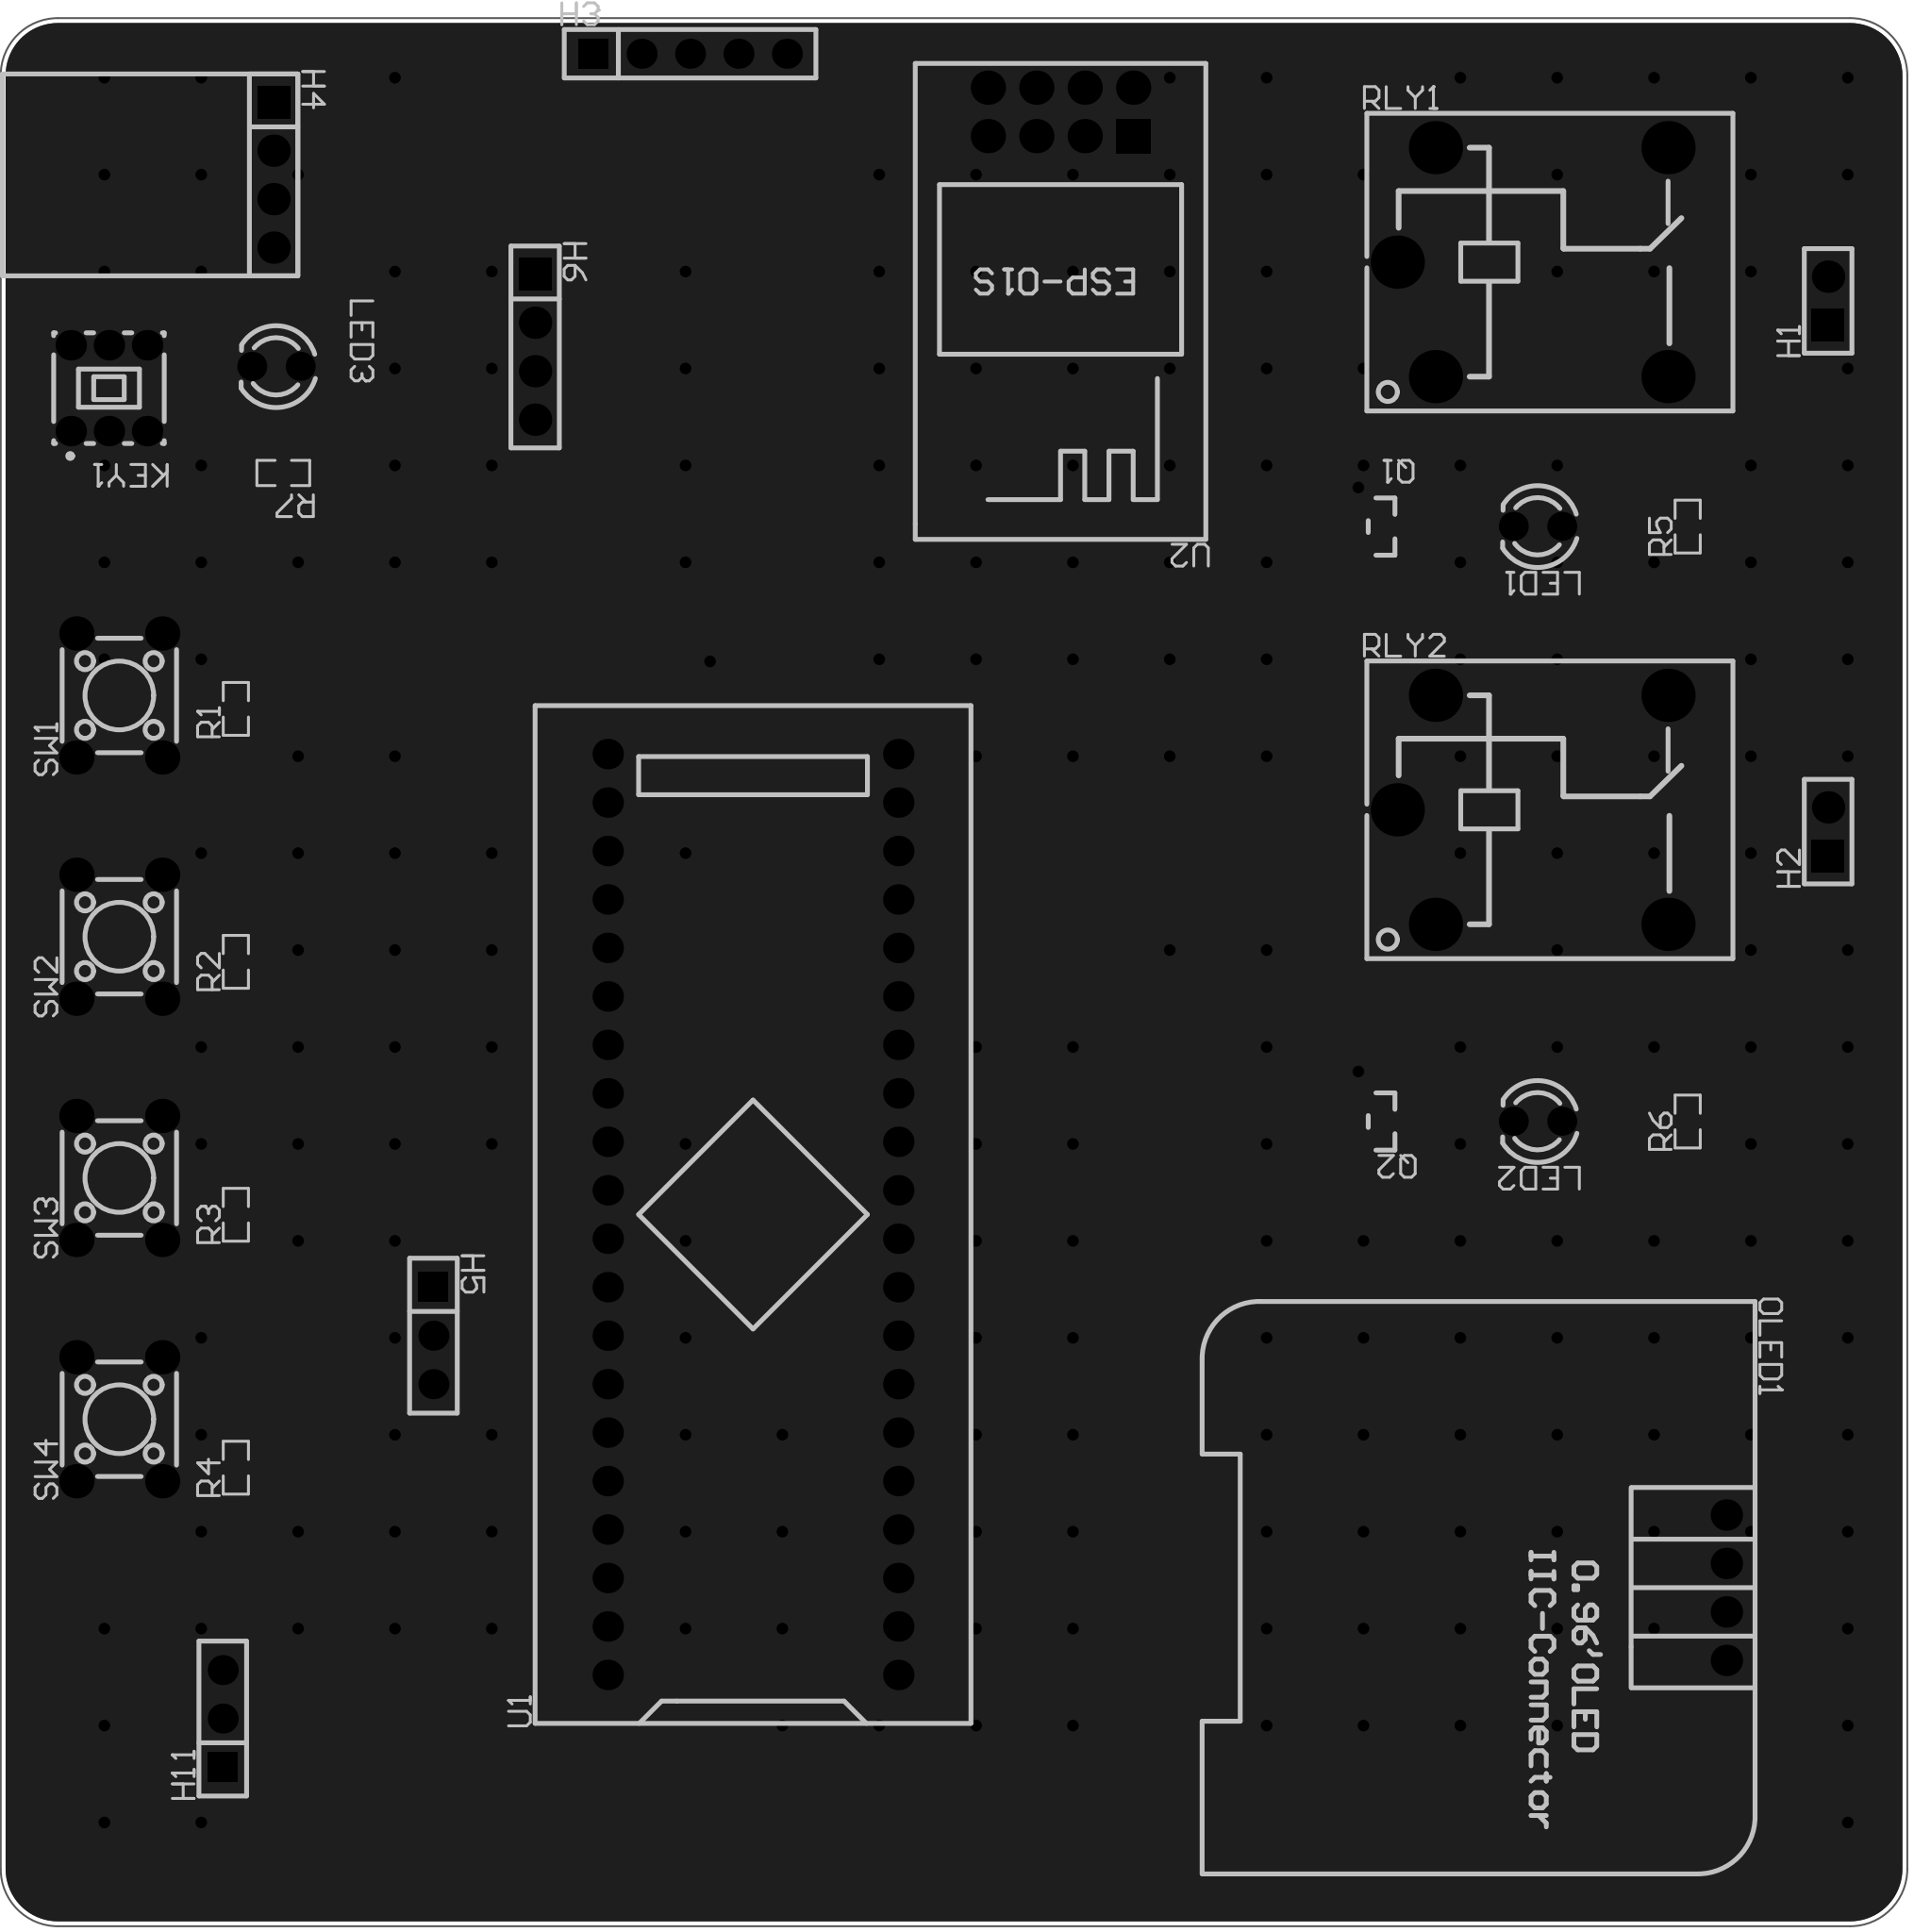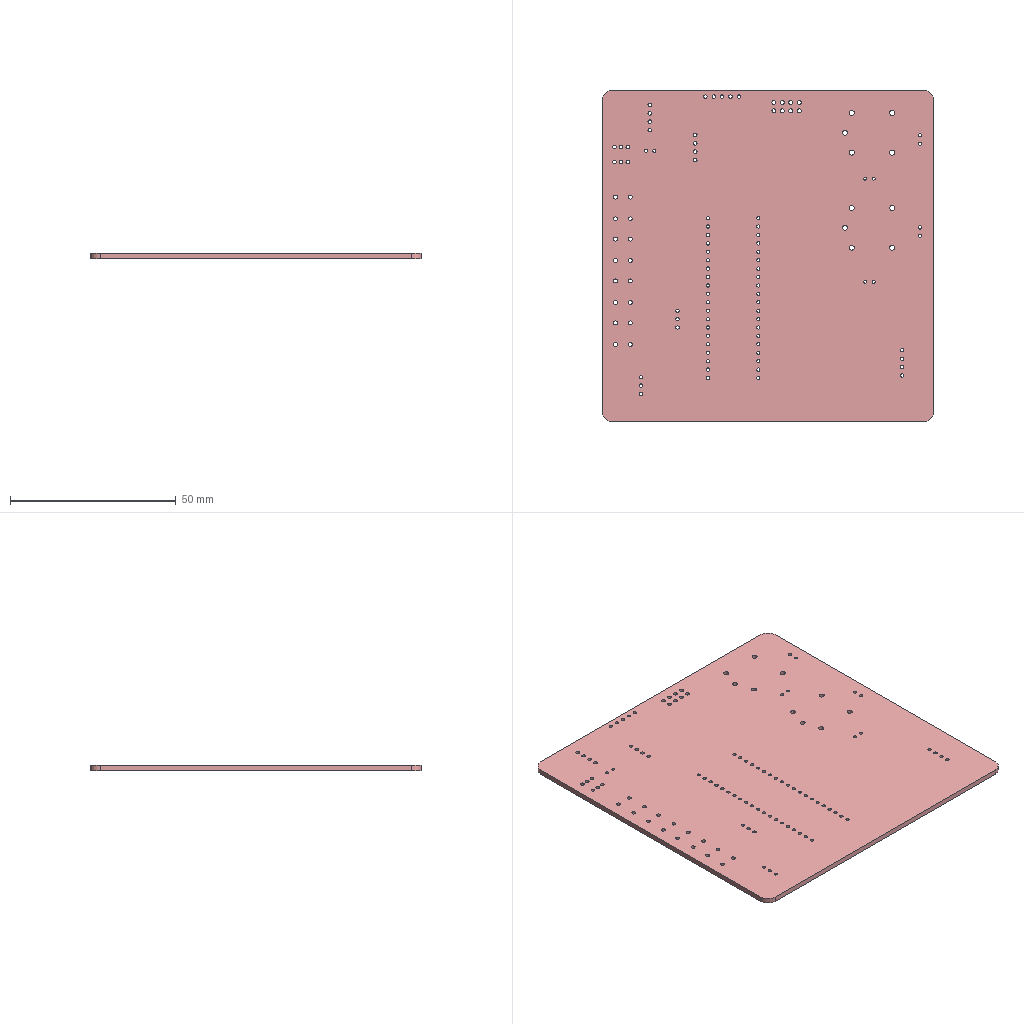Circuit board layout | Altium Designer | box 100 x 100 x 1.6 mm
Layer stack:
# Altium Designer layer stack of  (unit mm; dielectric type: 0 none, 1 core, 2 prepreg, 3 surface material)
index,name,kind,layer,copper_thickness_mm,dielectric_type,dielectric_thickness_mm,dielectric_material,dielectric_constant
0,Top Paste Mask Layer,other,,,,,,
1,Top Silkscreen Layer,other,,,,,,
2,Top Solder Mask Layer,dielectric,,,3,0.01,,3.3
3,Top Layer,copper,Top Layer,0.035,,,,
4,Dielectric1,dielectric,,,3,1.51,FR4,4.5
5,Bottom Layer,copper,Bottom Layer,0.035,,,,
6,Bottom Solder Mask Layer,dielectric,,,3,0.01,,3.3
7,Bottom Silkscreen Layer,other,,,,,,
8,Bottom Paste Mask Layer,other,,,,,,
# drill layer pairs: low layer,high layer
drill_pair,Top Layer,Bottom Layer
Part placement:
Designator,Comment,Layer,Footprint,Center-X(mm),Center-Y(mm),Rotation
H1,,TopLayer,HDR-TH_2P-P2.54-V-F,187.198,166.116,90
H2,,TopLayer,HDR-TH_2P-P2.54-V-F,187.198,138.303,90
H3,,TopLayer,HDR-TH_5P-P2.54-V-F,127.508,179.07,0
H4,,TopLayer,HDR-TH_4P-P2.54-V-F,105.664,172.72,270
H11,,TopLayer,HDR-TH_3P-P2.54-V-F,102.997,91.821,90
KEY1,Self-locking switch 5.8Z white-grey-white 260G,TopLayer,SW-TH_6P-L5.8-W5.8-P2.00-LS4.5-TR,97.028,161.544,180
LED3,,TopLayer,LED_TH-3mm,105.791,162.687,180
OLED1,,TopLayer,0.96OLED_4P,181.864,98.679,270
Q1,,TopLayer,S8050_SOT-23,163.777,154.29,180
Q2,,TopLayer,S8050_SOT-23,163.777,123.111,180
R1,10K,TopLayer,R0603,103.683,144.735,90
R2,10K,TopLayer,R0603,103.683,131.48,90
R3,10K,TopLayer,R0603,103.683,118.224,90
R4,10K,TopLayer,R0603,103.683,104.968,90
R5,1K,TopLayer,R0603,179.832,154.29,90
R6,1K,TopLayer,R0603,179.832,123.111,90
R7,1K,TopLayer,R0603,106.172,157.099,180
RLY1,SRD-05VDC-SL-C,TopLayer,RELAY-TH_SRD-XXVDC-XL-C,171.704,168.148,0
RLY2,SRD-05VDC-SL-C,TopLayer,RELAY-TH_SRD-XXVDC-XL-C,171.704,139.446,0
SW1,,TopLayer,SW-TH_4P-L6.0-W6.0-P4.50-LS6.5,97.572,145.439,90
SW2,,TopLayer,SW-TH_4P-L6.0-W6.0-P4.50-LS6.5,97.572,132.795,90
SW3,,TopLayer,SW-TH_4P-L6.0-W6.0-P4.50-LS6.5,97.572,120.152,90
SW4,,TopLayer,SW-TH_4P-L6.0-W6.0-P4.50-LS6.5,97.572,107.508,90
U1,STM32F103C8T6-Card,TopLayer,CONN-TH_L53.3-W22.9_STM32F103C8T6-CARD,130.81,118.237,90
U2,ESP-01S,TopLayer,WIFIM-TH_ESP-01S,146.939,176.022,180
LED1,,TopLayer,LED_TH-3mm,171.958,154.305,180
LED2,,TopLayer,LED_TH-3mm,171.958,123.126,180
H5,,TopLayer,HDR-TH_3P-P2.54-V-F,114.046,111.887,270
H6,,TopLayer,HDR-TH_4P-P2.54-V-F,119.38,163.703,270
Pad and via stacks:
# Altium Designer via and pad stacks of  (unit mm). Each distinct definition once, with the count of objects using it.
# via: kind,start_layer,end_layer,hole_mm,diameter_mm,mode(0 simple;1 top-mid-bottom;2 full stack),diameter_per_layer,count,example_net
# pad: kind,layer,hole_mm,hole_type(0 round;1 square;2 slot),plating,top_size,top_shape(1 round;2 rect;3 octagon;9 rounded rect),mid_size,bottom_size,mode,footprint,size_per_layer,count,example
pad,Multi-Layer,1,0,plated,1.7x1.7,2,1.7x1.7,1.7x1.7,0,HDR-TH_2P-P2.54-V-F,,2,H1.1
pad,Multi-Layer,1,0,plated,1.7x1.7,1,1.7x1.7,1.7x1.7,0,HDR-TH_2P-P2.54-V-F,,2,H1.2
pad,Multi-Layer,1.02,0,plated,1.575x1.575,1,1.575x1.575,1.575x1.575,0,HDR-TH_5P-P2.54-V-F,,4,H3.5
pad,Multi-Layer,1.02,0,plated,1.575x1.575,2,1.575x1.575,1.575x1.575,0,HDR-TH_5P-P2.54-V-F,,1,H3.1
pad,Multi-Layer,1.1,0,plated,1.7x1.7,2,1.7x1.7,1.7x1.7,0,HDR-TH_4P-P2.54-V-F,,2,H4.1
pad,Multi-Layer,1.1,0,plated,1.7x1.7,1,1.7x1.7,1.7x1.7,0,HDR-TH_4P-P2.54-V-F,,6,H4.2
pad,Multi-Layer,1.02,0,plated,1.575x1.575,1,1.575x1.575,1.575x1.575,0,HDR-TH_3P-P2.54-V-F,,4,H11.3
pad,Multi-Layer,1.02,0,plated,1.575x1.575,2,1.575x1.575,1.575x1.575,0,HDR-TH_3P-P2.54-V-F,,2,H11.1
pad,Multi-Layer,1.1,0,plated,1.6x1.6,1,1.6x1.6,1.6x1.6,0,SW-TH_6P-L5.8-W5.8-P2.00-LS4.5-TR,,6,KEY1.6
pad,Multi-Layer,0.9144,0,plated,1.524x1.524,1,1.524x1.524,1.524x1.524,0,LED_TH-3mm,,6,LED3.1
pad,Multi-Layer,1,0,plated,1.65x1.65,1,1.65x1.65,1.65x1.65,0,0.96OLED_4P,,4,OLED1.4
pad,Multi-Layer,1.524,0,plated,2.794x2.794,1,2.794x2.794,2.794x2.794,0,RELAY-TH_SRD-XXVDC-XL-C,,10,RLY1.2
pad,Multi-Layer,1.2,0,plated,1.8x1.8,1,1.8x1.8,1.8x1.8,0,SW-TH_4P-L6.0-W6.0-P4.50-LS6.5,,16,SW1.1
pad,Multi-Layer,1,0,plated,1.6x1.6,1,1.6x1.6,1.6x1.6,0,CONN-TH_L53.3-W22.9_STM32F103C8T6-CARD,,40,U1.1
pad,Multi-Layer,1.2,0,plated,1.8x1.8,2,1.8x1.8,1.8x1.8,0,WIFIM-TH_ESP-01S,,1,U2.1
pad,Multi-Layer,1.2,0,plated,1.8x1.8,1,1.8x1.8,1.8x1.8,0,WIFIM-TH_ESP-01S,,7,U2.2
pad,Top Layer,0,0,plated,1x0.8,2,1x0.8,1x0.8,0,S8050_SOT-23,,6,Q1.2
pad,Top Layer,0,0,plated,0.8065x0.864,2,0.8065x0.864,0.8065x0.864,0,R0603,,14,R1.2
via,Top Layer,Bottom Layer,0.3048,0.61,0,,222,VCC
Copper pours:
name,layer,net,type(0 solid;1 hatched;2 none)
Bottom Layer-GND,Bottom Layer,GND,0
Top Layer-GND,Top Layer,GND,0